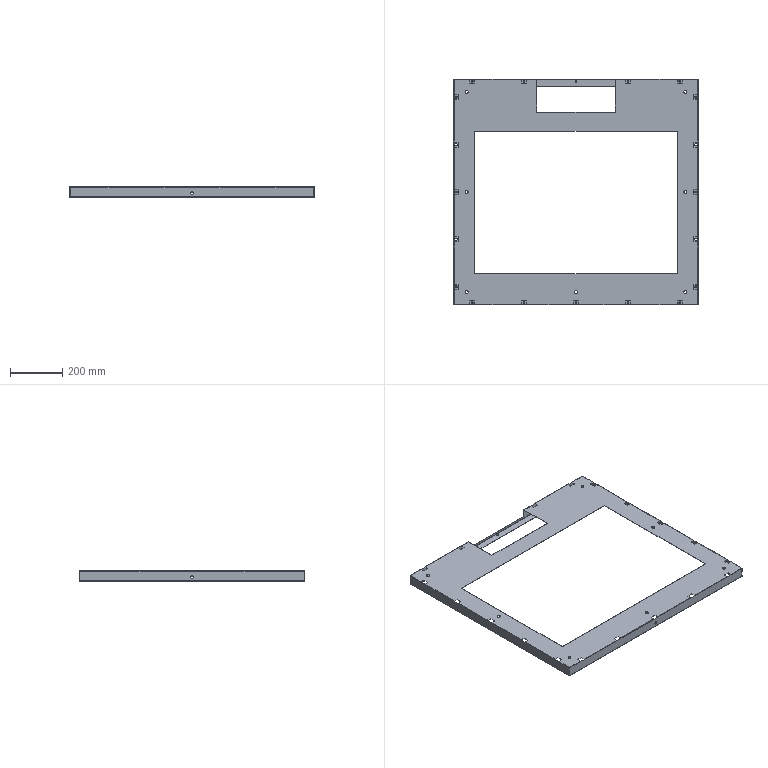Part | 1 solid | 384 faces | box 939 x 869 x 40 mm | volume 562183 mm3 | plane 242 | cylinder 126 | spline 16 | commonest cylinder face diameters 7 x50 0.4 x28 2.4 x28 11 x14 10 x6